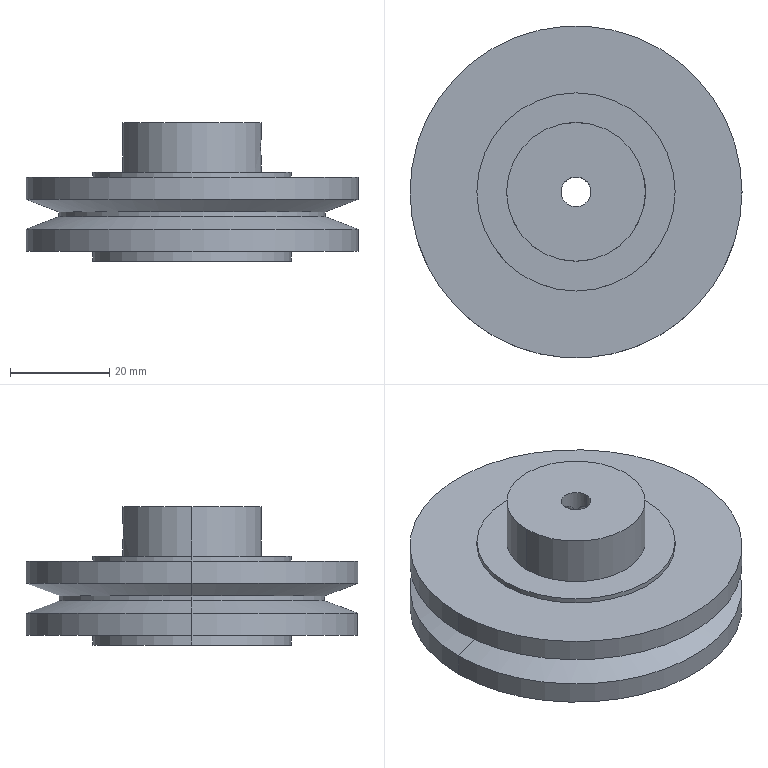Part | SolidWorks | features ICE 4, 3DProfileFeature 1, Extrusion 1, HoleWzd 1, RevCut 1 | 1 solid | 27 faces | box 67 x 67 x 28 mm | volume 57183 mm3 | cylinder 18 | plane 5 | cone 4 | commonest cylinder face diameters 4.2 x4 40 x4 67 x4 6 x2 28 x2 53.7 x2
STEP:
#1=CARTESIAN_POINT('',(0.,3.,18.9));
#2=VERTEX_POINT('',#1);
#3=CARTESIAN_POINT('',(0.,3.,23.1));
#4=VERTEX_POINT('',#3);
#5=CARTESIAN_POINT('',(0.,3.,18.9));
#6=CARTESIAN_POINT('',(-0.1421,3.,18.9));
#7=CARTESIAN_POINT('',(-0.2861,2.99,18.915));
#8=CARTESIAN_POINT('',(-0.5639,2.95,18.972));
#9=CARTESIAN_POINT('',(-0.6971,2.921,19.014));
#10=CARTESIAN_POINT('',(-1.081,2.811,19.178));
#11=CARTESIAN_POINT('',(-1.306,2.709,19.334));
#12=CARTESIAN_POINT('',(-1.585,2.549,19.616));
#13=CARTESIAN_POINT('',(-1.669,2.495,19.718));
#14=CARTESIAN_POINT('',(-1.817,2.389,19.939));
#15=CARTESIAN_POINT('',(-1.882,2.337,20.058));
#16=CARTESIAN_POINT('',(-1.987,2.249,20.307));
#17=CARTESIAN_POINT('',(-2.029,2.21,20.441));
#18=CARTESIAN_POINT('',(-2.086,2.157,20.717));
#19=CARTESIAN_POINT('',(-2.1,2.142,20.858));
#20=CARTESIAN_POINT('',(-2.1,2.143,21.147));
#21=CARTESIAN_POINT('',(-2.085,2.158,21.288));
#22=CARTESIAN_POINT('',(-2.028,2.211,21.564));
#23=CARTESIAN_POINT('',(-1.985,2.25,21.697));
#24=CARTESIAN_POINT('',(-1.827,2.384,22.071));
#25=CARTESIAN_POINT('',(-1.676,2.498,22.293));
#26=CARTESIAN_POINT('',(-1.395,2.658,22.575));
#27=CARTESIAN_POINT('',(-1.291,2.711,22.662));
#28=CARTESIAN_POINT('',(-1.069,2.805,22.812));
#29=CARTESIAN_POINT('',(-0.9512,2.848,22.877));
#30=CARTESIAN_POINT('',(-0.6975,2.921,22.986));
#31=CARTESIAN_POINT('',(-0.5613,2.95,23.028));
#32=CARTESIAN_POINT('',(-0.2858,2.99,23.085));
#33=CARTESIAN_POINT('',(-0.1442,3.,23.1));
#34=CARTESIAN_POINT('',(0.,3.,23.1));
#35=B_SPLINE_CURVE_WITH_KNOTS('',3,(#5,#6,#7,#8,#9,#10,#11,#12,#13,#14,#15,#16,#17,#18,#19,#20,#21,#22,#23,#24,#25,#26,#27,#28,#29,#30,#31,#32,#33,#34),.UNSPECIFIED.,.F.,.F.,(4,2,2,2,2,2,2,2,2,2,2,2,2,2,4),(0.006821,0.007247,0.007673,0.008524,0.00895,0.009376,0.009801,0.01023,0.01065,0.01108,0.01193,0.01236,0.01278,0.01321,0.01363),.UNSPECIFIED.);
#36=EDGE_CURVE('',#2,#4,#35,.T.);
#37=ORIENTED_EDGE('',*,*,#36,.F.);
#38=CARTESIAN_POINT('',(0.,14.,18.9));
#39=VERTEX_POINT('',#38);
#40=CARTESIAN_POINT('',(0.,14.,18.9));
#41=DIRECTION('',(0.,1.,0.));
#42=VECTOR('',#41,1000.);
#43=LINE('',#40,#42);
#44=EDGE_CURVE('',#2,#39,#43,.T.);
#45=ORIENTED_EDGE('',*,*,#44,.T.);
#46=CARTESIAN_POINT('',(0.,14.,23.1));
#47=VERTEX_POINT('',#46);
#48=CARTESIAN_POINT('',(0.,14.,23.1));
#49=CARTESIAN_POINT('',(-0.139,14.,23.1));
#50=CARTESIAN_POINT('',(-0.2756,13.998,23.086));
#51=CARTESIAN_POINT('',(-0.5443,13.99,23.033));
#52=CARTESIAN_POINT('',(-0.6777,13.984,22.992));
#53=CARTESIAN_POINT('',(-0.932,13.97,22.887));
#54=CARTESIAN_POINT('',(-1.053,13.961,22.822));
#55=CARTESIAN_POINT('',(-1.281,13.942,22.67));
#56=CARTESIAN_POINT('',(-1.389,13.931,22.581));
#57=CARTESIAN_POINT('',(-1.679,13.9,22.291));
#58=CARTESIAN_POINT('',(-1.835,13.88,22.057));
#59=CARTESIAN_POINT('',(-2.045,13.85,21.552));
#60=CARTESIAN_POINT('',(-2.1,13.842,21.275));
#61=CARTESIAN_POINT('',(-2.1,13.842,20.864));
#62=CARTESIAN_POINT('',(-2.086,13.844,20.724));
#63=CARTESIAN_POINT('',(-2.033,13.852,20.455));
#64=CARTESIAN_POINT('',(-1.993,13.858,20.324));
#65=CARTESIAN_POINT('',(-1.887,13.872,20.069));
#66=CARTESIAN_POINT('',(-1.822,13.881,19.947));
#67=CARTESIAN_POINT('',(-1.67,13.9,19.719));
#68=CARTESIAN_POINT('',(-1.583,13.911,19.613));
#69=CARTESIAN_POINT('',(-1.387,13.931,19.417));
#70=CARTESIAN_POINT('',(-1.281,13.942,19.331));
#71=CARTESIAN_POINT('',(-1.054,13.961,19.179));
#72=CARTESIAN_POINT('',(-0.9311,13.97,19.113));
#73=CARTESIAN_POINT('',(-0.6769,13.984,19.007));
#74=CARTESIAN_POINT('',(-0.546,13.99,18.968));
#75=CARTESIAN_POINT('',(-0.2765,13.998,18.914));
#76=CARTESIAN_POINT('',(-0.1372,14.,18.9));
#77=CARTESIAN_POINT('',(0.,14.,18.9));
#78=B_SPLINE_CURVE_WITH_KNOTS('',3,(#48,#49,#50,#51,#52,#53,#54,#55,#56,#57,#58,#59,#60,#61,#62,#63,#64,#65,#66,#67,#68,#69,#70,#71,#72,#73,#74,#75,#76,#77),.UNSPECIFIED.,.F.,.F.,(4,2,2,2,2,2,2,2,2,2,2,2,2,2,4),(0.,0.0004109,0.0008219,0.001233,0.001644,0.002466,0.003287,0.003698,0.004109,0.00452,0.004931,0.005342,0.005753,0.006164,0.006575),.UNSPECIFIED.);
#79=EDGE_CURVE('',#47,#39,#78,.T.);
#80=ORIENTED_EDGE('',*,*,#79,.F.);
#81=CARTESIAN_POINT('',(0.,14.,23.1));
#82=DIRECTION('',(0.,1.,0.));
#83=VECTOR('',#82,1000.);
#84=LINE('',#81,#83);
#85=EDGE_CURVE('',#4,#47,#84,.T.);
#86=ORIENTED_EDGE('',*,*,#85,.F.);
#87=EDGE_LOOP('',(#37,#45,#80,#86));
#88=FACE_OUTER_BOUND('',#87,.T.);
#89=CARTESIAN_POINT('',(0.,14.,21.));
#90=DIRECTION('',(0.,1.,0.));
#91=DIRECTION('',(0.,0.,1.));
#92=AXIS2_PLACEMENT_3D('',#89,#90,#91);
#93=CYLINDRICAL_SURFACE('',#92,2.1);
#94=ADVANCED_FACE('',(#88),#93,.F.);
#95=CARTESIAN_POINT('',(3.,0.,23.1));
#96=VERTEX_POINT('',#95);
#97=CARTESIAN_POINT('',(3.,0.,18.9));
#98=VERTEX_POINT('',#97);
#99=CARTESIAN_POINT('',(3.,0.,23.1));
#100=CARTESIAN_POINT('',(3.,-0.1421,23.1));
#101=CARTESIAN_POINT('',(2.99,-0.2861,23.085));
#102=CARTESIAN_POINT('',(2.95,-0.5639,23.028));
#103=CARTESIAN_POINT('',(2.921,-0.6971,22.986));
#104=CARTESIAN_POINT('',(2.811,-1.081,22.822));
#105=CARTESIAN_POINT('',(2.709,-1.306,22.666));
#106=CARTESIAN_POINT('',(2.549,-1.585,22.384));
#107=CARTESIAN_POINT('',(2.495,-1.669,22.282));
#108=CARTESIAN_POINT('',(2.389,-1.817,22.061));
#109=CARTESIAN_POINT('',(2.337,-1.882,21.942));
#110=CARTESIAN_POINT('',(2.249,-1.987,21.693));
#111=CARTESIAN_POINT('',(2.21,-2.029,21.559));
#112=CARTESIAN_POINT('',(2.157,-2.086,21.283));
#113=CARTESIAN_POINT('',(2.142,-2.1,21.142));
#114=CARTESIAN_POINT('',(2.143,-2.1,20.853));
#115=CARTESIAN_POINT('',(2.158,-2.085,20.712));
#116=CARTESIAN_POINT('',(2.211,-2.028,20.436));
#117=CARTESIAN_POINT('',(2.25,-1.985,20.303));
#118=CARTESIAN_POINT('',(2.384,-1.827,19.929));
#119=CARTESIAN_POINT('',(2.498,-1.676,19.707));
#120=CARTESIAN_POINT('',(2.658,-1.395,19.425));
#121=CARTESIAN_POINT('',(2.711,-1.291,19.338));
#122=CARTESIAN_POINT('',(2.805,-1.069,19.188));
#123=CARTESIAN_POINT('',(2.848,-0.9512,19.123));
#124=CARTESIAN_POINT('',(2.921,-0.6975,19.014));
#125=CARTESIAN_POINT('',(2.95,-0.5613,18.972));
#126=CARTESIAN_POINT('',(2.99,-0.2858,18.915));
#127=CARTESIAN_POINT('',(3.,-0.1442,18.9));
#128=CARTESIAN_POINT('',(3.,0.,18.9));
#129=B_SPLINE_CURVE_WITH_KNOTS('',3,(#99,#100,#101,#102,#103,#104,#105,#106,#107,#108,#109,#110,#111,#112,#113,#114,#115,#116,#117,#118,#119,#120,#121,#122,#123,#124,#125,#126,#127,#128),.UNSPECIFIED.,.F.,.F.,(4,2,2,2,2,2,2,2,2,2,2,2,2,2,4),(0.006821,0.007247,0.007673,0.008524,0.00895,0.009376,0.009801,0.01023,0.01065,0.01108,0.01193,0.01236,0.01278,0.01321,0.01363),.UNSPECIFIED.);
#130=EDGE_CURVE('',#96,#98,#129,.T.);
#131=ORIENTED_EDGE('',*,*,#130,.F.);
#132=CARTESIAN_POINT('',(14.,0.,23.1));
#133=VERTEX_POINT('',#132);
#134=CARTESIAN_POINT('',(14.,0.,23.1));
#135=DIRECTION('',(1.,0.,0.));
#136=VECTOR('',#135,1000.);
#137=LINE('',#134,#136);
#138=EDGE_CURVE('',#96,#133,#137,.T.);
#139=ORIENTED_EDGE('',*,*,#138,.T.);
#140=CARTESIAN_POINT('',(14.,0.,18.9));
#141=VERTEX_POINT('',#140);
#142=CARTESIAN_POINT('',(14.,0.,18.9));
#143=CARTESIAN_POINT('',(14.,-0.139,18.9));
#144=CARTESIAN_POINT('',(13.998,-0.2756,18.914));
#145=CARTESIAN_POINT('',(13.99,-0.5443,18.967));
#146=CARTESIAN_POINT('',(13.984,-0.6777,19.008));
#147=CARTESIAN_POINT('',(13.97,-0.932,19.113));
#148=CARTESIAN_POINT('',(13.961,-1.053,19.178));
#149=CARTESIAN_POINT('',(13.942,-1.281,19.33));
#150=CARTESIAN_POINT('',(13.931,-1.389,19.419));
#151=CARTESIAN_POINT('',(13.9,-1.679,19.709));
#152=CARTESIAN_POINT('',(13.88,-1.835,19.943));
#153=CARTESIAN_POINT('',(13.85,-2.045,20.448));
#154=CARTESIAN_POINT('',(13.842,-2.1,20.725));
#155=CARTESIAN_POINT('',(13.842,-2.1,21.136));
#156=CARTESIAN_POINT('',(13.844,-2.086,21.276));
#157=CARTESIAN_POINT('',(13.852,-2.033,21.545));
#158=CARTESIAN_POINT('',(13.858,-1.993,21.676));
#159=CARTESIAN_POINT('',(13.872,-1.887,21.931));
#160=CARTESIAN_POINT('',(13.881,-1.822,22.053));
#161=CARTESIAN_POINT('',(13.9,-1.67,22.281));
#162=CARTESIAN_POINT('',(13.911,-1.583,22.387));
#163=CARTESIAN_POINT('',(13.931,-1.387,22.583));
#164=CARTESIAN_POINT('',(13.942,-1.281,22.669));
#165=CARTESIAN_POINT('',(13.961,-1.054,22.821));
#166=CARTESIAN_POINT('',(13.97,-0.9311,22.887));
#167=CARTESIAN_POINT('',(13.984,-0.6769,22.993));
#168=CARTESIAN_POINT('',(13.99,-0.546,23.032));
#169=CARTESIAN_POINT('',(13.998,-0.2765,23.086));
#170=CARTESIAN_POINT('',(14.,-0.1372,23.1));
#171=CARTESIAN_POINT('',(14.,0.,23.1));
#172=B_SPLINE_CURVE_WITH_KNOTS('',3,(#142,#143,#144,#145,#146,#147,#148,#149,#150,#151,#152,#153,#154,#155,#156,#157,#158,#159,#160,#161,#162,#163,#164,#165,#166,#167,#168,#169,#170,#171),.UNSPECIFIED.,.F.,.F.,(4,2,2,2,2,2,2,2,2,2,2,2,2,2,4),(0.,0.0004109,0.0008219,0.001233,0.001644,0.002466,0.003287,0.003698,0.004109,0.00452,0.004931,0.005342,0.005753,0.006164,0.006575),.UNSPECIFIED.);
#173=EDGE_CURVE('',#141,#133,#172,.T.);
#174=ORIENTED_EDGE('',*,*,#173,.F.);
#175=CARTESIAN_POINT('',(14.,0.,18.9));
#176=DIRECTION('',(1.,0.,0.));
#177=VECTOR('',#176,1000.);
#178=LINE('',#175,#177);
#179=EDGE_CURVE('',#98,#141,#178,.T.);
#180=ORIENTED_EDGE('',*,*,#179,.F.);
#181=EDGE_LOOP('',(#131,#139,#174,#180));
#182=FACE_OUTER_BOUND('',#181,.T.);
#183=CARTESIAN_POINT('',(14.,0.,21.));
#184=DIRECTION('',(1.,0.,0.));
#185=DIRECTION('',(0.,0.,-1.));
#186=AXIS2_PLACEMENT_3D('',#183,#184,#185);
#187=CYLINDRICAL_SURFACE('',#186,2.1);
#188=ADVANCED_FACE('',(#182),#187,.F.);
#189=CARTESIAN_POINT('',(-26.85,0.,7.));
#190=VERTEX_POINT('',#189);
#191=CARTESIAN_POINT('',(26.85,0.,7.));
#192=VERTEX_POINT('',#191);
#193=CARTESIAN_POINT('',(0.,0.,7.));
#194=DIRECTION('',(0.,0.,-1.));
#195=DIRECTION('',(-1.,0.,0.));
#196=AXIS2_PLACEMENT_3D('',#193,#194,#195);
#197=CIRCLE('',#196,26.85);
#198=EDGE_CURVE('',#190,#192,#197,.T.);
#199=ORIENTED_EDGE('',*,*,#198,.T.);
#200=CARTESIAN_POINT('',(33.5,0.,4.5));
#201=VERTEX_POINT('',#200);
#202=CARTESIAN_POINT('',(26.85,0.,7.));
#203=DIRECTION('',(0.936,0.,-0.3519));
#204=VECTOR('',#203,1000.);
#205=LINE('',#202,#204);
#206=EDGE_CURVE('',#192,#201,#205,.T.);
#207=ORIENTED_EDGE('',*,*,#206,.T.);
#208=CARTESIAN_POINT('',(-33.5,0.,4.5));
#209=VERTEX_POINT('',#208);
#210=CARTESIAN_POINT('',(0.,0.,4.5));
#211=DIRECTION('',(0.,0.,-1.));
#212=DIRECTION('',(-1.,0.,0.));
#213=AXIS2_PLACEMENT_3D('',#210,#211,#212);
#214=CIRCLE('',#213,33.5);
#215=EDGE_CURVE('',#209,#201,#214,.T.);
#216=ORIENTED_EDGE('',*,*,#215,.F.);
#217=CARTESIAN_POINT('',(-26.85,0.,7.));
#218=DIRECTION('',(-0.936,0.,-0.3519));
#219=VECTOR('',#218,1000.);
#220=LINE('',#217,#219);
#221=EDGE_CURVE('',#190,#209,#220,.T.);
#222=ORIENTED_EDGE('',*,*,#221,.F.);
#223=EDGE_LOOP('',(#199,#207,#216,#222));
#224=FACE_OUTER_BOUND('',#223,.T.);
#225=CARTESIAN_POINT('',(0.,0.,7.));
#226=DIRECTION('',(0.,0.,-1.));
#227=DIRECTION('',(-1.,0.,0.));
#228=AXIS2_PLACEMENT_3D('',#225,#226,#227);
#229=CONICAL_SURFACE('',#228,26.85,1.211);
#230=ADVANCED_FACE('',(#224),#229,.T.);
#231=CARTESIAN_POINT('',(-26.85,0.,8.));
#232=VERTEX_POINT('',#231);
#233=CARTESIAN_POINT('',(26.85,0.,8.));
#234=VERTEX_POINT('',#233);
#235=CARTESIAN_POINT('',(0.,0.,8.));
#236=DIRECTION('',(0.,0.,-1.));
#237=DIRECTION('',(-1.,0.,0.));
#238=AXIS2_PLACEMENT_3D('',#235,#236,#237);
#239=CIRCLE('',#238,26.85);
#240=EDGE_CURVE('',#232,#234,#239,.T.);
#241=ORIENTED_EDGE('',*,*,#240,.T.);
#242=CARTESIAN_POINT('',(26.85,0.,0.));
#243=DIRECTION('',(0.,0.,-1.));
#244=VECTOR('',#243,1000.);
#245=LINE('',#242,#244);
#246=EDGE_CURVE('',#234,#192,#245,.T.);
#247=ORIENTED_EDGE('',*,*,#246,.T.);
#248=ORIENTED_EDGE('',*,*,#198,.F.);
#249=CARTESIAN_POINT('',(-26.85,0.,0.));
#250=DIRECTION('',(0.,0.,-1.));
#251=VECTOR('',#250,1000.);
#252=LINE('',#249,#251);
#253=EDGE_CURVE('',#232,#190,#252,.T.);
#254=ORIENTED_EDGE('',*,*,#253,.F.);
#255=EDGE_LOOP('',(#241,#247,#248,#254));
#256=FACE_OUTER_BOUND('',#255,.T.);
#257=CARTESIAN_POINT('',(0.,0.,0.));
#258=DIRECTION('',(0.,0.,-1.));
#259=DIRECTION('',(-1.,0.,0.));
#260=AXIS2_PLACEMENT_3D('',#257,#258,#259);
#261=CYLINDRICAL_SURFACE('',#260,26.85);
#262=ADVANCED_FACE('',(#256),#261,.T.);
#263=ORIENTED_EDGE('',*,*,#240,.F.);
#264=CARTESIAN_POINT('',(-33.5,0.,10.5));
#265=VERTEX_POINT('',#264);
#266=CARTESIAN_POINT('',(-33.5,0.,10.5));
#267=DIRECTION('',(-0.936,0.,0.3519));
#268=VECTOR('',#267,1000.);
#269=LINE('',#266,#268);
#270=EDGE_CURVE('',#232,#265,#269,.T.);
#271=ORIENTED_EDGE('',*,*,#270,.T.);
#272=CARTESIAN_POINT('',(33.5,0.,10.5));
#273=VERTEX_POINT('',#272);
#274=CARTESIAN_POINT('',(0.,0.,10.5));
#275=DIRECTION('',(0.,0.,-1.));
#276=DIRECTION('',(-1.,0.,0.));
#277=AXIS2_PLACEMENT_3D('',#274,#275,#276);
#278=CIRCLE('',#277,33.5);
#279=EDGE_CURVE('',#265,#273,#278,.T.);
#280=ORIENTED_EDGE('',*,*,#279,.T.);
#281=CARTESIAN_POINT('',(33.5,0.,10.5));
#282=DIRECTION('',(0.936,0.,0.3519));
#283=VECTOR('',#282,1000.);
#284=LINE('',#281,#283);
#285=EDGE_CURVE('',#234,#273,#284,.T.);
#286=ORIENTED_EDGE('',*,*,#285,.F.);
#287=EDGE_LOOP('',(#263,#271,#280,#286));
#288=FACE_OUTER_BOUND('',#287,.T.);
#289=CARTESIAN_POINT('',(0.,0.,10.5));
#290=DIRECTION('',(0.,0.,1.));
#291=DIRECTION('',(1.,0.,0.));
#292=AXIS2_PLACEMENT_3D('',#289,#290,#291);
#293=CONICAL_SURFACE('',#292,33.5,1.211);
#294=ADVANCED_FACE('',(#288),#293,.T.);
#295=CARTESIAN_POINT('',(-3.,0.,-2.));
#296=VERTEX_POINT('',#295);
#297=CARTESIAN_POINT('',(3.,0.,-2.));
#298=VERTEX_POINT('',#297);
#299=CARTESIAN_POINT('',(0.,0.,-2.));
#300=DIRECTION('',(0.,0.,1.));
#301=DIRECTION('',(1.,0.,0.));
#302=AXIS2_PLACEMENT_3D('',#299,#300,#301);
#303=CIRCLE('',#302,3.);
#304=EDGE_CURVE('',#296,#298,#303,.T.);
#305=ORIENTED_EDGE('',*,*,#304,.F.);
#306=CARTESIAN_POINT('',(-3.,0.,26.));
#307=VERTEX_POINT('',#306);
#308=CARTESIAN_POINT('',(-3.,0.,-2.));
#309=DIRECTION('',(0.,0.,1.));
#310=VECTOR('',#309,1000.);
#311=LINE('',#308,#310);
#312=EDGE_CURVE('',#296,#307,#311,.T.);
#313=ORIENTED_EDGE('',*,*,#312,.T.);
#314=CARTESIAN_POINT('',(3.,0.,26.));
#315=VERTEX_POINT('',#314);
#316=CARTESIAN_POINT('',(0.,0.,26.));
#317=DIRECTION('',(0.,0.,1.));
#318=DIRECTION('',(1.,0.,0.));
#319=AXIS2_PLACEMENT_3D('',#316,#317,#318);
#320=CIRCLE('',#319,3.);
#321=EDGE_CURVE('',#307,#315,#320,.T.);
#322=ORIENTED_EDGE('',*,*,#321,.T.);
#323=CARTESIAN_POINT('',(3.,0.,-2.));
#324=DIRECTION('',(0.,0.,1.));
#325=VECTOR('',#324,1000.);
#326=LINE('',#323,#325);
#327=EDGE_CURVE('',#96,#315,#326,.T.);
#328=ORIENTED_EDGE('',*,*,#327,.F.);
#329=ORIENTED_EDGE('',*,*,#130,.T.);
#330=CARTESIAN_POINT('',(3.,0.,-2.));
#331=DIRECTION('',(0.,0.,1.));
#332=VECTOR('',#331,1000.);
#333=LINE('',#330,#332);
#334=EDGE_CURVE('',#298,#98,#333,.T.);
#335=ORIENTED_EDGE('',*,*,#334,.F.);
#336=EDGE_LOOP('',(#305,#313,#322,#328,#329,#335));
#337=FACE_OUTER_BOUND('',#336,.T.);
#338=CARTESIAN_POINT('',(0.,0.,-2.));
#339=DIRECTION('',(0.,0.,1.));
#340=DIRECTION('',(1.,0.,0.));
#341=AXIS2_PLACEMENT_3D('',#338,#339,#340);
#342=CYLINDRICAL_SURFACE('',#341,3.);
#343=ADVANCED_FACE('',(#337),#342,.F.);
#344=ORIENTED_EDGE('',*,*,#79,.T.);
#345=CARTESIAN_POINT('',(0.,14.,18.9));
#346=CARTESIAN_POINT('',(0.2742,14.,18.9));
#347=CARTESIAN_POINT('',(0.5509,13.991,18.955));
#348=CARTESIAN_POINT('',(0.93,13.97,19.112));
#349=CARTESIAN_POINT('',(1.052,13.961,19.177));
#350=CARTESIAN_POINT('',(1.282,13.942,19.331));
#351=CARTESIAN_POINT('',(1.387,13.931,19.417));
#352=CARTESIAN_POINT('',(1.581,13.911,19.611));
#353=CARTESIAN_POINT('',(1.669,13.9,19.719));
#354=CARTESIAN_POINT('',(1.822,13.881,19.946));
#355=CARTESIAN_POINT('',(1.886,13.872,20.067));
#356=CARTESIAN_POINT('',(1.992,13.858,20.321));
#357=CARTESIAN_POINT('',(2.033,13.852,20.454));
#358=CARTESIAN_POINT('',(2.086,13.844,20.723));
#359=CARTESIAN_POINT('',(2.1,13.842,20.86));
#360=CARTESIAN_POINT('',(2.1,13.842,21.137));
#361=CARTESIAN_POINT('',(2.087,13.844,21.274));
#362=CARTESIAN_POINT('',(2.033,13.852,21.543));
#363=CARTESIAN_POINT('',(1.993,13.858,21.676));
#364=CARTESIAN_POINT('',(1.888,13.872,21.93));
#365=CARTESIAN_POINT('',(1.823,13.881,22.051));
#366=CARTESIAN_POINT('',(1.671,13.9,22.279));
#367=CARTESIAN_POINT('',(1.583,13.911,22.387));
#368=CARTESIAN_POINT('',(1.293,13.942,22.677));
#369=CARTESIAN_POINT('',(1.059,13.962,22.834));
#370=CARTESIAN_POINT('',(0.5539,13.991,23.044));
#371=CARTESIAN_POINT('',(0.2779,14.,23.1));
#372=CARTESIAN_POINT('',(0.,14.,23.1));
#373=B_SPLINE_CURVE_WITH_KNOTS('',3,(#345,#346,#347,#348,#349,#350,#351,#352,#353,#354,#355,#356,#357,#358,#359,#360,#361,#362,#363,#364,#365,#366,#367,#368,#369,#370,#371,#372),.UNSPECIFIED.,.F.,.F.,(4,2,2,2,2,2,2,2,2,2,2,2,2,4),(0.006575,0.007396,0.007807,0.008218,0.008629,0.00904,0.009451,0.009861,0.01027,0.01068,0.01109,0.0115,0.01233,0.01315),.UNSPECIFIED.);
#374=EDGE_CURVE('',#39,#47,#373,.T.);
#375=ORIENTED_EDGE('',*,*,#374,.T.);
#376=EDGE_LOOP('',(#344,#375));
#377=FACE_BOUND('',#376,.T.);
#378=CARTESIAN_POINT('',(14.,0.,26.));
#379=VERTEX_POINT('',#378);
#380=CARTESIAN_POINT('',(-14.,0.,26.));
#381=VERTEX_POINT('',#380);
#382=CARTESIAN_POINT('',(0.,0.,26.));
#383=DIRECTION('',(0.,0.,1.));
#384=DIRECTION('',(1.,0.,0.));
#385=AXIS2_PLACEMENT_3D('',#382,#383,#384);
#386=CIRCLE('',#385,14.);
#387=EDGE_CURVE('',#379,#381,#386,.T.);
#388=ORIENTED_EDGE('',*,*,#387,.F.);
#389=CARTESIAN_POINT('',(14.,0.,26.));
#390=DIRECTION('',(0.,0.,-1.));
#391=VECTOR('',#390,1000.);
#392=LINE('',#389,#391);
#393=EDGE_CURVE('',#379,#133,#392,.T.);
#394=ORIENTED_EDGE('',*,*,#393,.T.);
#395=CARTESIAN_POINT('',(14.,0.,23.1));
#396=CARTESIAN_POINT('',(14.,0.2742,23.1));
#397=CARTESIAN_POINT('',(13.991,0.5509,23.045));
#398=CARTESIAN_POINT('',(13.97,0.93,22.888));
#399=CARTESIAN_POINT('',(13.961,1.052,22.823));
#400=CARTESIAN_POINT('',(13.942,1.282,22.669));
#401=CARTESIAN_POINT('',(13.931,1.387,22.583));
#402=CARTESIAN_POINT('',(13.911,1.581,22.389));
#403=CARTESIAN_POINT('',(13.9,1.669,22.281));
#404=CARTESIAN_POINT('',(13.881,1.822,22.054));
#405=CARTESIAN_POINT('',(13.872,1.886,21.933));
#406=CARTESIAN_POINT('',(13.858,1.992,21.679));
#407=CARTESIAN_POINT('',(13.852,2.033,21.546));
#408=CARTESIAN_POINT('',(13.844,2.086,21.277));
#409=CARTESIAN_POINT('',(13.842,2.1,21.14));
#410=CARTESIAN_POINT('',(13.842,2.1,20.863));
#411=CARTESIAN_POINT('',(13.844,2.087,20.726));
#412=CARTESIAN_POINT('',(13.852,2.033,20.457));
#413=CARTESIAN_POINT('',(13.858,1.993,20.324));
#414=CARTESIAN_POINT('',(13.872,1.888,20.07));
#415=CARTESIAN_POINT('',(13.881,1.823,19.949));
#416=CARTESIAN_POINT('',(13.9,1.671,19.721));
#417=CARTESIAN_POINT('',(13.911,1.583,19.613));
#418=CARTESIAN_POINT('',(13.942,1.293,19.323));
#419=CARTESIAN_POINT('',(13.962,1.059,19.166));
#420=CARTESIAN_POINT('',(13.991,0.5539,18.956));
#421=CARTESIAN_POINT('',(14.,0.2779,18.9));
#422=CARTESIAN_POINT('',(14.,0.,18.9));
#423=B_SPLINE_CURVE_WITH_KNOTS('',3,(#395,#396,#397,#398,#399,#400,#401,#402,#403,#404,#405,#406,#407,#408,#409,#410,#411,#412,#413,#414,#415,#416,#417,#418,#419,#420,#421,#422),.UNSPECIFIED.,.F.,.F.,(4,2,2,2,2,2,2,2,2,2,2,2,2,4),(0.006575,0.007396,0.007807,0.008218,0.008629,0.00904,0.009451,0.009861,0.01027,0.01068,0.01109,0.0115,0.01233,0.01315),.UNSPECIFIED.);
#424=EDGE_CURVE('',#133,#141,#423,.T.);
#425=ORIENTED_EDGE('',*,*,#424,.T.);
#426=CARTESIAN_POINT('',(14.,0.,16.));
#427=VERTEX_POINT('',#426);
#428=CARTESIAN_POINT('',(14.,0.,26.));
#429=DIRECTION('',(0.,0.,-1.));
#430=VECTOR('',#429,1000.);
#431=LINE('',#428,#430);
#432=EDGE_CURVE('',#141,#427,#431,.T.);
#433=ORIENTED_EDGE('',*,*,#432,.T.);
#434=CARTESIAN_POINT('',(-14.,0.,16.));
#435=VERTEX_POINT('',#434);
#436=CARTESIAN_POINT('',(0.,0.,16.));
#437=DIRECTION('',(0.,0.,1.));
#438=DIRECTION('',(1.,0.,0.));
#439=AXIS2_PLACEMENT_3D('',#436,#437,#438);
#440=CIRCLE('',#439,14.);
#441=EDGE_CURVE('',#427,#435,#440,.T.);
#442=ORIENTED_EDGE('',*,*,#441,.T.);
#443=CARTESIAN_POINT('',(-14.,0.,26.));
#444=DIRECTION('',(0.,0.,-1.));
#445=VECTOR('',#444,1000.);
#446=LINE('',#443,#445);
#447=EDGE_CURVE('',#381,#435,#446,.T.);
#448=ORIENTED_EDGE('',*,*,#447,.F.);
#449=EDGE_LOOP('',(#388,#394,#425,#433,#442,#448));
#450=FACE_OUTER_BOUND('',#449,.T.);
#451=CARTESIAN_POINT('',(0.,0.,26.));
#452=DIRECTION('',(0.,0.,-1.));
#453=DIRECTION('',(-1.,0.,0.));
#454=AXIS2_PLACEMENT_3D('',#451,#452,#453);
#455=CYLINDRICAL_SURFACE('',#454,14.);
#456=ADVANCED_FACE('',(#377,#450),#455,.T.);
#457=CARTESIAN_POINT('',(20.,0.,16.));
#458=VERTEX_POINT('',#457);
#459=CARTESIAN_POINT('',(-20.,0.,16.));
#460=VERTEX_POINT('',#459);
#461=CARTESIAN_POINT('',(0.,0.,16.));
#462=DIRECTION('',(0.,0.,1.));
#463=DIRECTION('',(1.,0.,0.));
#464=AXIS2_PLACEMENT_3D('',#461,#462,#463);
#465=CIRCLE('',#464,20.);
#466=EDGE_CURVE('',#458,#460,#465,.T.);
#467=ORIENTED_EDGE('',*,*,#466,.F.);
#468=CARTESIAN_POINT('',(20.,0.,15.));
#469=VERTEX_POINT('',#468);
#470=CARTESIAN_POINT('',(20.,0.,16.));
#471=DIRECTION('',(0.,0.,-1.));
#472=VECTOR('',#471,1000.);
#473=LINE('',#470,#472);
#474=EDGE_CURVE('',#458,#469,#473,.T.);
#475=ORIENTED_EDGE('',*,*,#474,.T.);
#476=CARTESIAN_POINT('',(-20.,0.,15.));
#477=VERTEX_POINT('',#476);
#478=CARTESIAN_POINT('',(0.,0.,15.));
#479=DIRECTION('',(0.,0.,1.));
#480=DIRECTION('',(1.,0.,0.));
#481=AXIS2_PLACEMENT_3D('',#478,#479,#480);
#482=CIRCLE('',#481,20.);
#483=EDGE_CURVE('',#469,#477,#482,.T.);
#484=ORIENTED_EDGE('',*,*,#483,.T.);
#485=CARTESIAN_POINT('',(-20.,0.,16.));
#486=DIRECTION('',(0.,0.,-1.));
#487=VECTOR('',#486,1000.);
#488=LINE('',#485,#487);
#489=EDGE_CURVE('',#460,#477,#488,.T.);
#490=ORIENTED_EDGE('',*,*,#489,.F.);
#491=EDGE_LOOP('',(#467,#475,#484,#490));
#492=FACE_OUTER_BOUND('',#491,.T.);
#493=CARTESIAN_POINT('',(0.,0.,16.));
#494=DIRECTION('',(0.,0.,-1.));
#495=DIRECTION('',(-1.,0.,0.));
#496=AXIS2_PLACEMENT_3D('',#493,#494,#495);
#497=CYLINDRICAL_SURFACE('',#496,20.);
#498=ADVANCED_FACE('',(#492),#497,.T.);
#499=CARTESIAN_POINT('',(-20.,0.,-2.));
#500=VERTEX_POINT('',#499);
#501=CARTESIAN_POINT('',(20.,0.,-2.));
#502=VERTEX_POINT('',#501);
#503=CARTESIAN_POINT('',(0.,0.,-2.));
#504=DIRECTION('',(0.,0.,-1.));
#505=DIRECTION('',(-1.,0.,0.));
#506=AXIS2_PLACEMENT_3D('',#503,#504,#505);
#507=CIRCLE('',#506,20.);
#508=EDGE_CURVE('',#500,#502,#507,.T.);
#509=ORIENTED_EDGE('',*,*,#508,.F.);
#510=CARTESIAN_POINT('',(-20.,0.,0.));
#511=VERTEX_POINT('',#510);
#512=CARTESIAN_POINT('',(-20.,0.,-2.));
#513=DIRECTION('',(0.,0.,1.));
#514=VECTOR('',#513,1000.);
#515=LINE('',#512,#514);
#516=EDGE_CURVE('',#500,#511,#515,.T.);
#517=ORIENTED_EDGE('',*,*,#516,.T.);
#518=CARTESIAN_POINT('',(20.,0.,0.));
#519=VERTEX_POINT('',#518);
#520=CARTESIAN_POINT('',(0.,0.,0.));
#521=DIRECTION('',(0.,0.,-1.));
#522=DIRECTION('',(-1.,0.,0.));
#523=AXIS2_PLACEMENT_3D('',#520,#521,#522);
#524=CIRCLE('',#523,20.);
#525=EDGE_CURVE('',#511,#519,#524,.T.);
#526=ORIENTED_EDGE('',*,*,#525,.T.);
#527=CARTESIAN_POINT('',(20.,0.,-2.));
#528=DIRECTION('',(0.,0.,1.));
#529=VECTOR('',#528,1000.);
#530=LINE('',#527,#529);
#531=EDGE_CURVE('',#502,#519,#530,.T.);
#532=ORIENTED_EDGE('',*,*,#531,.F.);
#533=EDGE_LOOP('',(#509,#517,#526,#532));
#534=FACE_OUTER_BOUND('',#533,.T.);
#535=CARTESIAN_POINT('',(0.,0.,-2.));
#536=DIRECTION('',(0.,0.,1.));
#537=DIRECTION('',(1.,0.,0.));
#538=AXIS2_PLACEMENT_3D('',#535,#536,#537);
#539=CYLINDRICAL_SURFACE('',#538,20.);
#540=ADVANCED_FACE('',(#534),#539,.T.);
#541=ORIENTED_EDGE('',*,*,#215,.T.);
#542=CARTESIAN_POINT('',(33.5,0.,0.));
#543=VERTEX_POINT('',#542);
#544=CARTESIAN_POINT('',(33.5,0.,15.));
#545=DIRECTION('',(0.,0.,-1.));
#546=VECTOR('',#545,1000.);
#547=LINE('',#544,#546);
#548=EDGE_CURVE('',#201,#543,#547,.T.);
#549=ORIENTED_EDGE('',*,*,#548,.T.);
#550=CARTESIAN_POINT('',(-33.5,0.,0.));
#551=VERTEX_POINT('',#550);
#552=CARTESIAN_POINT('',(0.,0.,0.));
#553=DIRECTION('',(0.,0.,1.));
#554=DIRECTION('',(1.,0.,0.));
#555=AXIS2_PLACEMENT_3D('',#552,#553,#554);
#556=CIRCLE('',#555,33.5);
#557=EDGE_CURVE('',#543,#551,#556,.T.);
#558=ORIENTED_EDGE('',*,*,#557,.T.);
#559=CARTESIAN_POINT('',(-33.5,0.,15.));
#560=DIRECTION('',(0.,0.,-1.));
#561=VECTOR('',#560,1000.);
#562=LINE('',#559,#561);
#563=EDGE_CURVE('',#209,#551,#562,.T.);
#564=ORIENTED_EDGE('',*,*,#563,.F.);
#565=EDGE_LOOP('',(#541,#549,#558,#564));
#566=FACE_OUTER_BOUND('',#565,.T.);
#567=CARTESIAN_POINT('',(0.,0.,15.));
#568=DIRECTION('',(0.,0.,-1.));
#569=DIRECTION('',(-1.,0.,0.));
#570=AXIS2_PLACEMENT_3D('',#567,#568,#569);
#571=CYLINDRICAL_SURFACE('',#570,33.5);
#572=ADVANCED_FACE('',(#566),#571,.T.);
#573=CARTESIAN_POINT('',(33.5,0.,15.));
#574=VERTEX_POINT('',#573);
#575=CARTESIAN_POINT('',(-33.5,0.,15.));
#576=VERTEX_POINT('',#575);
#577=CARTESIAN_POINT('',(0.,0.,15.));
#578=DIRECTION('',(0.,0.,1.));
#579=DIRECTION('',(1.,0.,0.));
#580=AXIS2_PLACEMENT_3D('',#577,#578,#579);
#581=CIRCLE('',#580,33.5);
#582=EDGE_CURVE('',#574,#576,#581,.T.);
#583=ORIENTED_EDGE('',*,*,#582,.F.);
#584=CARTESIAN_POINT('',(33.5,0.,15.));
#585=DIRECTION('',(0.,0.,-1.));
#586=VECTOR('',#585,1000.);
#587=LINE('',#584,#586);
#588=EDGE_CURVE('',#574,#273,#587,.T.);
#589=ORIENTED_EDGE('',*,*,#588,.T.);
#590=ORIENTED_EDGE('',*,*,#279,.F.);
#591=CARTESIAN_POINT('',(-33.5,0.,15.));
#592=DIRECTION('',(0.,0.,-1.));
#593=VECTOR('',#592,1000.);
#594=LINE('',#591,#593);
#595=EDGE_CURVE('',#576,#265,#594,.T.);
#596=ORIENTED_EDGE('',*,*,#595,.F.);
#597=EDGE_LOOP('',(#583,#589,#590,#596));
#598=FACE_OUTER_BOUND('',#597,.T.);
#599=CARTESIAN_POINT('',(0.,0.,15.));
#600=DIRECTION('',(0.,0.,-1.));
#601=DIRECTION('',(-1.,0.,0.));
#602=AXIS2_PLACEMENT_3D('',#599,#600,#601);
#603=CYLINDRICAL_SURFACE('',#602,33.5);
#604=ADVANCED_FACE('',(#598),#603,.T.);
#605=ORIENTED_EDGE('',*,*,#588,.F.);
#606=CARTESIAN_POINT('',(0.,0.,15.));
#607=DIRECTION('',(0.,0.,1.));
#608=DIRECTION('',(1.,0.,0.));
#609=AXIS2_PLACEMENT_3D('',#606,#607,#608);
#610=CIRCLE('',#609,33.5);
#611=EDGE_CURVE('',#576,#574,#610,.T.);
#612=ORIENTED_EDGE('',*,*,#611,.F.);
#613=ORIENTED_EDGE('',*,*,#595,.T.);
#614=CARTESIAN_POINT('',(0.,0.,10.5));
#615=DIRECTION('',(0.,0.,-1.));
#616=DIRECTION('',(-1.,0.,0.));
#617=AXIS2_PLACEMENT_3D('',#614,#615,#616);
#618=CIRCLE('',#617,33.5);
#619=EDGE_CURVE('',#273,#265,#618,.T.);
#620=ORIENTED_EDGE('',*,*,#619,.F.);
#621=EDGE_LOOP('',(#605,#612,#613,#620));
#622=FACE_OUTER_BOUND('',#621,.T.);
#623=CARTESIAN_POINT('',(0.,0.,15.));
#624=DIRECTION('',(0.,0.,-1.));
#625=DIRECTION('',(-1.,0.,0.));
#626=AXIS2_PLACEMENT_3D('',#623,#624,#625);
#627=CYLINDRICAL_SURFACE('',#626,33.5);
#628=ADVANCED_FACE('',(#622),#627,.T.);
#629=ORIENTED_EDGE('',*,*,#548,.F.);
#630=CARTESIAN_POINT('',(0.,0.,4.5));
#631=DIRECTION('',(0.,0.,-1.));
#632=DIRECTION('',(-1.,0.,0.));
#633=AXIS2_PLACEMENT_3D('',#630,#631,#632);
#634=CIRCLE('',#633,33.5);
#635=EDGE_CURVE('',#201,#209,#634,.T.);
#636=ORIENTED_EDGE('',*,*,#635,.T.);
#637=ORIENTED_EDGE('',*,*,#563,.T.);
#638=CARTESIAN_POINT('',(0.,0.,0.));
#639=DIRECTION('',(0.,0.,1.));
#640=DIRECTION('',(1.,0.,0.));
#641=AXIS2_PLACEMENT_3D('',#638,#639,#640);
#642=CIRCLE('',#641,33.5);
#643=EDGE_CURVE('',#551,#543,#642,.T.);
#644=ORIENTED_EDGE('',*,*,#643,.T.);
#645=EDGE_LOOP('',(#629,#636,#637,#644));
#646=FACE_OUTER_BOUND('',#645,.T.);
#647=CARTESIAN_POINT('',(0.,0.,15.));
#648=DIRECTION('',(0.,0.,-1.));
#649=DIRECTION('',(-1.,0.,0.));
#650=AXIS2_PLACEMENT_3D('',#647,#648,#649);
#651=CYLINDRICAL_SURFACE('',#650,33.5);
#652=ADVANCED_FACE('',(#646),#651,.T.);
#653=CARTESIAN_POINT('',(0.,0.,15.));
#654=DIRECTION('',(0.,0.,1.));
#655=DIRECTION('',(1.,0.,0.));
#656=AXIS2_PLACEMENT_3D('',#653,#654,#655);
#657=CIRCLE('',#656,20.);
#658=EDGE_CURVE('',#477,#469,#657,.T.);
#659=ORIENTED_EDGE('',*,*,#658,.F.);
#660=ORIENTED_EDGE('',*,*,#483,.F.);
#661=EDGE_LOOP('',(#659,#660));
#662=FACE_BOUND('',#661,.T.);
#663=ORIENTED_EDGE('',*,*,#611,.T.);
#664=ORIENTED_EDGE('',*,*,#582,.T.);
#665=EDGE_LOOP('',(#663,#664));
#666=FACE_OUTER_BOUND('',#665,.T.);
#667=CARTESIAN_POINT('',(0.,0.,15.));
#668=DIRECTION('',(0.,0.,1.));
#669=DIRECTION('',(1.,0.,0.));
#670=AXIS2_PLACEMENT_3D('',#667,#668,#669);
#671=PLANE('',#670);
#672=ADVANCED_FACE('',(#662,#666),#671,.T.);
#673=CARTESIAN_POINT('',(0.,0.,0.));
#674=DIRECTION('',(0.,0.,-1.));
#675=DIRECTION('',(-1.,0.,0.));
#676=AXIS2_PLACEMENT_3D('',#673,#674,#675);
#677=CIRCLE('',#676,20.);
#678=EDGE_CURVE('',#519,#511,#677,.T.);
#679=ORIENTED_EDGE('',*,*,#678,.F.);
#680=ORIENTED_EDGE('',*,*,#525,.F.);
#681=EDGE_LOOP('',(#679,#680));
#682=FACE_BOUND('',#681,.T.);
#683=ORIENTED_EDGE('',*,*,#643,.F.);
#684=ORIENTED_EDGE('',*,*,#557,.F.);
#685=EDGE_LOOP('',(#683,#684));
#686=FACE_OUTER_BOUND('',#685,.T.);
#687=CARTESIAN_POINT('',(0.,0.,0.));
#688=DIRECTION('',(0.,0.,1.));
#689=DIRECTION('',(1.,0.,0.));
#690=AXIS2_PLACEMENT_3D('',#687,#688,#689);
#691=PLANE('',#690);
#692=ADVANCED_FACE('',(#682,#686),#691,.F.);
#693=ORIENTED_EDGE('',*,*,#516,.F.);
#694=CARTESIAN_POINT('',(0.,0.,-2.));
#695=DIRECTION('',(0.,0.,-1.));
#696=DIRECTION('',(-1.,0.,0.));
#697=AXIS2_PLACEMENT_3D('',#694,#695,#696);
#698=CIRCLE('',#697,20.);
#699=EDGE_CURVE('',#502,#500,#698,.T.);
#700=ORIENTED_EDGE('',*,*,#699,.F.);
#701=ORIENTED_EDGE('',*,*,#531,.T.);
#702=ORIENTED_EDGE('',*,*,#678,.T.);
#703=EDGE_LOOP('',(#693,#700,#701,#702));
#704=FACE_OUTER_BOUND('',#703,.T.);
#705=CARTESIAN_POINT('',(0.,0.,-2.));
#706=DIRECTION('',(0.,0.,1.));
#707=DIRECTION('',(1.,0.,0.));
#708=AXIS2_PLACEMENT_3D('',#705,#706,#707);
#709=CYLINDRICAL_SURFACE('',#708,20.);
#710=ADVANCED_FACE('',(#704),#709,.T.);
#711=CARTESIAN_POINT('',(0.,0.,-2.));
#712=DIRECTION('',(0.,0.,1.));
#713=DIRECTION('',(1.,0.,0.));
#714=AXIS2_PLACEMENT_3D('',#711,#712,#713);
#715=CIRCLE('',#714,3.);
#716=EDGE_CURVE('',#298,#296,#715,.T.);
#717=ORIENTED_EDGE('',*,*,#716,.T.);
#718=ORIENTED_EDGE('',*,*,#304,.T.);
#719=EDGE_LOOP('',(#717,#718));
#720=FACE_BOUND('',#719,.T.);
#721=ORIENTED_EDGE('',*,*,#699,.T.);
#722=ORIENTED_EDGE('',*,*,#508,.T.);
#723=EDGE_LOOP('',(#721,#722));
#724=FACE_OUTER_BOUND('',#723,.T.);
#725=CARTESIAN_POINT('',(0.,0.,-2.));
#726=DIRECTION('',(0.,0.,-1.));
#727=DIRECTION('',(-1.,0.,0.));
#728=AXIS2_PLACEMENT_3D('',#725,#726,#727);
#729=PLANE('',#728);
#730=ADVANCED_FACE('',(#720,#724),#729,.T.);
#731=ORIENTED_EDGE('',*,*,#474,.F.);
#732=CARTESIAN_POINT('',(0.,0.,16.));
#733=DIRECTION('',(0.,0.,1.));
#734=DIRECTION('',(1.,0.,0.));
#735=AXIS2_PLACEMENT_3D('',#732,#733,#734);
#736=CIRCLE('',#735,20.);
#737=EDGE_CURVE('',#460,#458,#736,.T.);
#738=ORIENTED_EDGE('',*,*,#737,.F.);
#739=ORIENTED_EDGE('',*,*,#489,.T.);
#740=ORIENTED_EDGE('',*,*,#658,.T.);
#741=EDGE_LOOP('',(#731,#738,#739,#740));
#742=FACE_OUTER_BOUND('',#741,.T.);
#743=CARTESIAN_POINT('',(0.,0.,16.));
#744=DIRECTION('',(0.,0.,-1.));
#745=DIRECTION('',(-1.,0.,0.));
#746=AXIS2_PLACEMENT_3D('',#743,#744,#745);
#747=CYLINDRICAL_SURFACE('',#746,20.);
#748=ADVANCED_FACE('',(#742),#747,.T.);
#749=CARTESIAN_POINT('',(0.,0.,16.));
#750=DIRECTION('',(0.,0.,1.));
#751=DIRECTION('',(1.,0.,0.));
#752=AXIS2_PLACEMENT_3D('',#749,#750,#751);
#753=CIRCLE('',#752,14.);
#754=EDGE_CURVE('',#435,#427,#753,.T.);
#755=ORIENTED_EDGE('',*,*,#754,.F.);
#756=ORIENTED_EDGE('',*,*,#441,.F.);
#757=EDGE_LOOP('',(#755,#756));
#758=FACE_BOUND('',#757,.T.);
#759=ORIENTED_EDGE('',*,*,#737,.T.);
#760=ORIENTED_EDGE('',*,*,#466,.T.);
#761=EDGE_LOOP('',(#759,#760));
#762=FACE_OUTER_BOUND('',#761,.T.);
#763=CARTESIAN_POINT('',(0.,0.,16.));
#764=DIRECTION('',(0.,0.,1.));
#765=DIRECTION('',(1.,0.,0.));
#766=AXIS2_PLACEMENT_3D('',#763,#764,#765);
#767=PLANE('',#766);
#768=ADVANCED_FACE('',(#758,#762),#767,.T.);
#769=CARTESIAN_POINT('',(0.,0.,26.));
#770=DIRECTION('',(0.,0.,1.));
#771=DIRECTION('',(1.,0.,0.));
#772=AXIS2_PLACEMENT_3D('',#769,#770,#771);
#773=CIRCLE('',#772,3.);
#774=EDGE_CURVE('',#315,#307,#773,.T.);
#775=ORIENTED_EDGE('',*,*,#774,.F.);
#776=ORIENTED_EDGE('',*,*,#321,.F.);
#777=EDGE_LOOP('',(#775,#776));
#778=FACE_BOUND('',#777,.T.);
#779=CARTESIAN_POINT('',(0.,0.,26.));
#780=DIRECTION('',(0.,0.,1.));
#781=DIRECTION('',(1.,0.,0.));
#782=AXIS2_PLACEMENT_3D('',#779,#780,#781);
#783=CIRCLE('',#782,14.);
#784=EDGE_CURVE('',#381,#379,#783,.T.);
#785=ORIENTED_EDGE('',*,*,#784,.T.);
#786=ORIENTED_EDGE('',*,*,#387,.T.);
#787=EDGE_LOOP('',(#785,#786));
#788=FACE_OUTER_BOUND('',#787,.T.);
#789=CARTESIAN_POINT('',(0.,0.,26.));
#790=DIRECTION('',(0.,0.,1.));
#791=DIRECTION('',(1.,0.,0.));
#792=AXIS2_PLACEMENT_3D('',#789,#790,#791);
#793=PLANE('',#792);
#794=ADVANCED_FACE('',(#778,#788),#793,.T.);
#795=ORIENTED_EDGE('',*,*,#393,.F.);
#796=ORIENTED_EDGE('',*,*,#784,.F.);
#797=ORIENTED_EDGE('',*,*,#447,.T.);
#798=ORIENTED_EDGE('',*,*,#754,.T.);
#799=ORIENTED_EDGE('',*,*,#432,.F.);
#800=ORIENTED_EDGE('',*,*,#173,.T.);
#801=EDGE_LOOP('',(#795,#796,#797,#798,#799,#800));
#802=FACE_OUTER_BOUND('',#801,.T.);
#803=CARTESIAN_POINT('',(0.,0.,26.));
#804=DIRECTION('',(0.,0.,-1.));
#805=DIRECTION('',(-1.,0.,0.));
#806=AXIS2_PLACEMENT_3D('',#803,#804,#805);
#807=CYLINDRICAL_SURFACE('',#806,14.);
#808=ADVANCED_FACE('',(#802),#807,.T.);
#809=ORIENTED_EDGE('',*,*,#312,.F.);
#810=ORIENTED_EDGE('',*,*,#716,.F.);
#811=ORIENTED_EDGE('',*,*,#334,.T.);
#812=CARTESIAN_POINT('',(3.,0.,18.9));
#813=CARTESIAN_POINT('',(3.,0.1444,18.9));
#814=CARTESIAN_POINT('',(2.99,0.2856,18.915));
#815=CARTESIAN_POINT('',(2.95,0.5619,18.972));
#816=CARTESIAN_POINT('',(2.921,0.6979,19.015));
#817=CARTESIAN_POINT('',(2.812,1.078,19.177));
#818=CARTESIAN_POINT('',(2.71,1.304,19.333));
#819=CARTESIAN_POINT('',(2.55,1.584,19.615));
#820=CARTESIAN_POINT('',(2.495,1.669,19.718));
#821=CARTESIAN_POINT('',(2.389,1.816,19.938));
#822=CARTESIAN_POINT('',(2.339,1.88,20.054));
#823=CARTESIAN_POINT('',(2.25,1.986,20.304));
#824=CARTESIAN_POINT('',(2.211,2.028,20.438));
#825=CARTESIAN_POINT('',(2.157,2.085,20.712));
#826=CARTESIAN_POINT('',(2.142,2.1,20.857));
#827=CARTESIAN_POINT('',(2.142,2.1,21.142));
#828=CARTESIAN_POINT('',(2.157,2.086,21.284));
#829=CARTESIAN_POINT('',(2.211,2.028,21.562));
#830=CARTESIAN_POINT('',(2.249,1.987,21.693));
#831=CARTESIAN_POINT('',(2.384,1.827,22.071));
#832=CARTESIAN_POINT('',(2.496,1.679,22.29));
#833=CARTESIAN_POINT('',(2.657,1.397,22.574));
#834=CARTESIAN_POINT('',(2.709,1.295,22.659));
#835=CARTESIAN_POINT('',(2.804,1.073,22.81));
#836=CARTESIAN_POINT('',(2.848,0.9532,22.876));
#837=CARTESIAN_POINT('',(2.921,0.6976,22.986));
#838=CARTESIAN_POINT('',(2.95,0.5645,23.028));
#839=CARTESIAN_POINT('',(2.99,0.2866,23.085));
#840=CARTESIAN_POINT('',(3.,0.1423,23.1));
#841=CARTESIAN_POINT('',(3.,0.,23.1));
#842=B_SPLINE_CURVE_WITH_KNOTS('',3,(#812,#813,#814,#815,#816,#817,#818,#819,#820,#821,#822,#823,#824,#825,#826,#827,#828,#829,#830,#831,#832,#833,#834,#835,#836,#837,#838,#839,#840,#841),.UNSPECIFIED.,.F.,.F.,(4,2,2,2,2,2,2,2,2,2,2,2,2,2,4),(0.,0.0004263,0.0008526,0.001705,0.002132,0.002558,0.002984,0.003411,0.003837,0.004263,0.005116,0.005542,0.005969,0.006395,0.006821),.UNSPECIFIED.);
#843=EDGE_CURVE('',#98,#96,#842,.T.);
#844=ORIENTED_EDGE('',*,*,#843,.T.);
#845=ORIENTED_EDGE('',*,*,#327,.T.);
#846=ORIENTED_EDGE('',*,*,#774,.T.);
#847=EDGE_LOOP('',(#809,#810,#811,#844,#845,#846));
#848=FACE_OUTER_BOUND('',#847,.T.);
#849=CARTESIAN_POINT('',(0.,3.,23.1));
#850=CARTESIAN_POINT('',(0.1444,3.,23.1));
#851=CARTESIAN_POINT('',(0.2856,2.99,23.085));
#852=CARTESIAN_POINT('',(0.5619,2.95,23.028));
#853=CARTESIAN_POINT('',(0.6979,2.921,22.985));
#854=CARTESIAN_POINT('',(1.078,2.812,22.823));
#855=CARTESIAN_POINT('',(1.304,2.71,22.667));
#856=CARTESIAN_POINT('',(1.584,2.55,22.385));
#857=CARTESIAN_POINT('',(1.669,2.495,22.282));
#858=CARTESIAN_POINT('',(1.816,2.389,22.062));
#859=CARTESIAN_POINT('',(1.88,2.339,21.946));
#860=CARTESIAN_POINT('',(1.986,2.25,21.696));
#861=CARTESIAN_POINT('',(2.028,2.211,21.562));
#862=CARTESIAN_POINT('',(2.085,2.157,21.288));
#863=CARTESIAN_POINT('',(2.1,2.142,21.143));
#864=CARTESIAN_POINT('',(2.1,2.142,20.858));
#865=CARTESIAN_POINT('',(2.086,2.157,20.716));
#866=CARTESIAN_POINT('',(2.028,2.211,20.438));
#867=CARTESIAN_POINT('',(1.987,2.249,20.307));
#868=CARTESIAN_POINT('',(1.827,2.384,19.929));
#869=CARTESIAN_POINT('',(1.679,2.496,19.71));
#870=CARTESIAN_POINT('',(1.397,2.657,19.426));
#871=CARTESIAN_POINT('',(1.295,2.709,19.341));
#872=CARTESIAN_POINT('',(1.073,2.804,19.19));
#873=CARTESIAN_POINT('',(0.9532,2.848,19.124));
#874=CARTESIAN_POINT('',(0.6976,2.921,19.014));
#875=CARTESIAN_POINT('',(0.5645,2.95,18.972));
#876=CARTESIAN_POINT('',(0.2866,2.99,18.915));
#877=CARTESIAN_POINT('',(0.1423,3.,18.9));
#878=CARTESIAN_POINT('',(0.,3.,18.9));
#879=B_SPLINE_CURVE_WITH_KNOTS('',3,(#849,#850,#851,#852,#853,#854,#855,#856,#857,#858,#859,#860,#861,#862,#863,#864,#865,#866,#867,#868,#869,#870,#871,#872,#873,#874,#875,#876,#877,#878),.UNSPECIFIED.,.F.,.F.,(4,2,2,2,2,2,2,2,2,2,2,2,2,2,4),(0.,0.0004263,0.0008526,0.001705,0.002132,0.002558,0.002984,0.003411,0.003837,0.004263,0.005116,0.005542,0.005969,0.006395,0.006821),.UNSPECIFIED.);
#880=EDGE_CURVE('',#4,#2,#879,.T.);
#881=ORIENTED_EDGE('',*,*,#880,.T.);
#882=ORIENTED_EDGE('',*,*,#36,.T.);
#883=EDGE_LOOP('',(#881,#882));
#884=FACE_BOUND('',#883,.T.);
#885=CARTESIAN_POINT('',(0.,0.,-2.));
#886=DIRECTION('',(0.,0.,1.));
#887=DIRECTION('',(1.,0.,0.));
#888=AXIS2_PLACEMENT_3D('',#885,#886,#887);
#889=CYLINDRICAL_SURFACE('',#888,3.);
#890=ADVANCED_FACE('',(#848,#884),#889,.F.);
#891=ORIENTED_EDGE('',*,*,#270,.F.);
#892=CARTESIAN_POINT('',(0.,0.,8.));
#893=DIRECTION('',(0.,0.,-1.));
#894=DIRECTION('',(-1.,0.,0.));
#895=AXIS2_PLACEMENT_3D('',#892,#893,#894);
#896=CIRCLE('',#895,26.85);
#897=EDGE_CURVE('',#234,#232,#896,.T.);
#898=ORIENTED_EDGE('',*,*,#897,.F.);
#899=ORIENTED_EDGE('',*,*,#285,.T.);
#900=ORIENTED_EDGE('',*,*,#619,.T.);
#901=EDGE_LOOP('',(#891,#898,#899,#900));
#902=FACE_OUTER_BOUND('',#901,.T.);
#903=CARTESIAN_POINT('',(0.,0.,10.5));
#904=DIRECTION('',(0.,0.,1.));
#905=DIRECTION('',(1.,0.,0.));
#906=AXIS2_PLACEMENT_3D('',#903,#904,#905);
#907=CONICAL_SURFACE('',#906,33.5,1.211);
#908=ADVANCED_FACE('',(#902),#907,.T.);
#909=ORIENTED_EDGE('',*,*,#246,.F.);
#910=ORIENTED_EDGE('',*,*,#897,.T.);
#911=ORIENTED_EDGE('',*,*,#253,.T.);
#912=CARTESIAN_POINT('',(0.,0.,7.));
#913=DIRECTION('',(0.,0.,-1.));
#914=DIRECTION('',(-1.,0.,0.));
#915=AXIS2_PLACEMENT_3D('',#912,#913,#914);
#916=CIRCLE('',#915,26.85);
#917=EDGE_CURVE('',#192,#190,#916,.T.);
#918=ORIENTED_EDGE('',*,*,#917,.F.);
#919=EDGE_LOOP('',(#909,#910,#911,#918));
#920=FACE_OUTER_BOUND('',#919,.T.);
#921=CARTESIAN_POINT('',(0.,0.,0.));
#922=DIRECTION('',(0.,0.,-1.));
#923=DIRECTION('',(-1.,0.,0.));
#924=AXIS2_PLACEMENT_3D('',#921,#922,#923);
#925=CYLINDRICAL_SURFACE('',#924,26.85);
#926=ADVANCED_FACE('',(#920),#925,.T.);
#927=ORIENTED_EDGE('',*,*,#206,.F.);
#928=ORIENTED_EDGE('',*,*,#917,.T.);
#929=ORIENTED_EDGE('',*,*,#221,.T.);
#930=ORIENTED_EDGE('',*,*,#635,.F.);
#931=EDGE_LOOP('',(#927,#928,#929,#930));
#932=FACE_OUTER_BOUND('',#931,.T.);
#933=CARTESIAN_POINT('',(0.,0.,7.));
#934=DIRECTION('',(0.,0.,-1.));
#935=DIRECTION('',(-1.,0.,0.));
#936=AXIS2_PLACEMENT_3D('',#933,#934,#935);
#937=CONICAL_SURFACE('',#936,26.85,1.211);
#938=ADVANCED_FACE('',(#932),#937,.T.);
#939=ORIENTED_EDGE('',*,*,#138,.F.);
#940=ORIENTED_EDGE('',*,*,#843,.F.);
#941=ORIENTED_EDGE('',*,*,#179,.T.);
#942=ORIENTED_EDGE('',*,*,#424,.F.);
#943=EDGE_LOOP('',(#939,#940,#941,#942));
#944=FACE_OUTER_BOUND('',#943,.T.);
#945=CARTESIAN_POINT('',(14.,0.,21.));
#946=DIRECTION('',(1.,0.,0.));
#947=DIRECTION('',(0.,0.,-1.));
#948=AXIS2_PLACEMENT_3D('',#945,#946,#947);
#949=CYLINDRICAL_SURFACE('',#948,2.1);
#950=ADVANCED_FACE('',(#944),#949,.F.);
#951=ORIENTED_EDGE('',*,*,#44,.F.);
#952=ORIENTED_EDGE('',*,*,#880,.F.);
#953=ORIENTED_EDGE('',*,*,#85,.T.);
#954=ORIENTED_EDGE('',*,*,#374,.F.);
#955=EDGE_LOOP('',(#951,#952,#953,#954));
#956=FACE_OUTER_BOUND('',#955,.T.);
#957=CARTESIAN_POINT('',(0.,14.,21.));
#958=DIRECTION('',(0.,1.,0.));
#959=DIRECTION('',(0.,0.,1.));
#960=AXIS2_PLACEMENT_3D('',#957,#958,#959);
#961=CYLINDRICAL_SURFACE('',#960,2.1);
#962=ADVANCED_FACE('',(#956),#961,.F.);
#963=CLOSED_SHELL('',(#94,#188,#230,#262,#294,#343,#456,#498,#540,#572,#604,#628,#652,#672,#692,#710,#730,#748,#768,#794,#808,#890,#908,#926,#938,#950,#962));
#964=MANIFOLD_SOLID_BREP('',#963);
#965=CARTESIAN_POINT('',(0.,0.,0.));
#966=DIRECTION('',(0.,0.,1.));
#967=DIRECTION('',(1.,0.,0.));
#968=AXIS2_PLACEMENT_3D('',#965,#966,#967);
#969=(LENGTH_UNIT()NAMED_UNIT(*)SI_UNIT(.MILLI.,.METRE.));
#970=UNCERTAINTY_MEASURE_WITH_UNIT(LENGTH_MEASURE(0.00001),#969,'','');
#971=(NAMED_UNIT(*)PLANE_ANGLE_UNIT()SI_UNIT($,.RADIAN.));
#972=(NAMED_UNIT(*)SI_UNIT($,.STERADIAN.)SOLID_ANGLE_UNIT());
#973=(GEOMETRIC_REPRESENTATION_CONTEXT(3)GLOBAL_UNCERTAINTY_ASSIGNED_CONTEXT((#970))GLOBAL_UNIT_ASSIGNED_CONTEXT((#969,#971,#972))REPRESENTATION_CONTEXT('',''));
#974=ADVANCED_BREP_SHAPE_REPRESENTATION('',(#964,#968),#973);